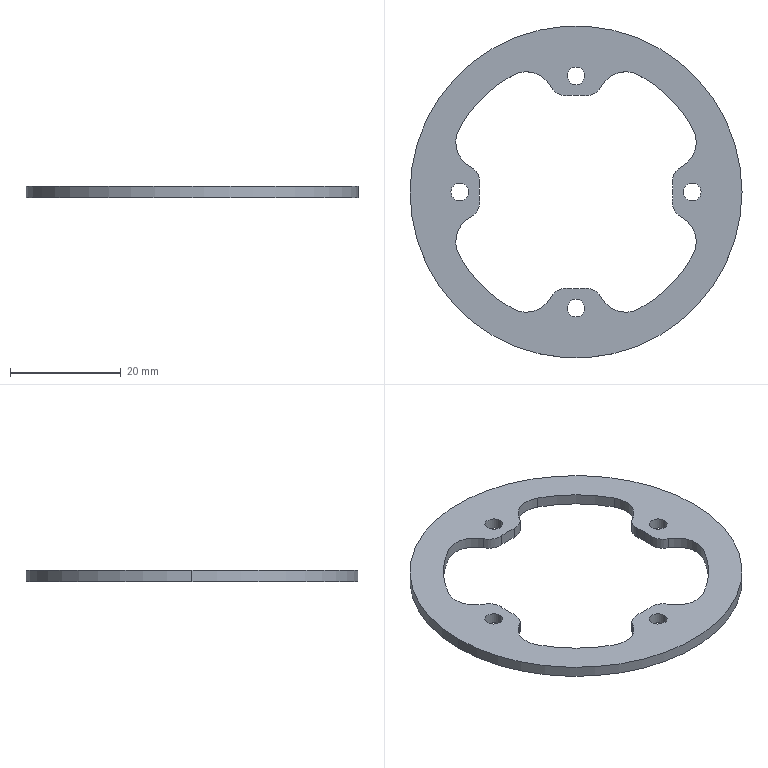Part | SolidWorks | features ICE 3, Extrusion 1, Fillet 1 | 1 solid | 41 faces | box 60 x 60 x 2 mm | volume 2571 mm3 | cylinder 39 | plane 2 | commonest cylinder face diameters 6 x10 10 x10 3.2 x8 35 x5 48 x4 60 x2
STEP:
#1=CARTESIAN_POINT('',(-17.412,1.896,0.));
#2=VERTEX_POINT('',#1);
#3=CARTESIAN_POINT('',(-17.425,1.619,0.));
#4=VERTEX_POINT('',#3);
#5=CARTESIAN_POINT('',(-20.412,1.896,0.));
#6=DIRECTION('',(0.,0.,-1.));
#7=DIRECTION('',(1.,0.,0.));
#8=AXIS2_PLACEMENT_3D('',#5,#6,#7);
#9=CIRCLE('',#8,3.);
#10=EDGE_CURVE('',#2,#4,#9,.T.);
#11=ORIENTED_EDGE('',*,*,#10,.F.);
#12=CARTESIAN_POINT('',(-17.412,1.896,2.));
#13=VERTEX_POINT('',#12);
#14=CARTESIAN_POINT('',(-17.412,1.896,2.));
#15=DIRECTION('',(0.,0.,1.));
#16=VECTOR('',#15,1000.);
#17=LINE('',#14,#16);
#18=EDGE_CURVE('',#2,#13,#17,.T.);
#19=ORIENTED_EDGE('',*,*,#18,.T.);
#20=CARTESIAN_POINT('',(-17.425,1.619,2.));
#21=VERTEX_POINT('',#20);
#22=CARTESIAN_POINT('',(-20.412,1.896,2.));
#23=DIRECTION('',(0.,0.,1.));
#24=DIRECTION('',(1.,0.,0.));
#25=AXIS2_PLACEMENT_3D('',#22,#23,#24);
#26=CIRCLE('',#25,3.);
#27=EDGE_CURVE('',#21,#13,#26,.T.);
#28=ORIENTED_EDGE('',*,*,#27,.F.);
#29=CARTESIAN_POINT('',(-17.425,1.619,-8.));
#30=DIRECTION('',(0.,0.,1.));
#31=VECTOR('',#30,1000.);
#32=LINE('',#29,#31);
#33=EDGE_CURVE('',#4,#21,#32,.T.);
#34=ORIENTED_EDGE('',*,*,#33,.F.);
#35=EDGE_LOOP('',(#11,#19,#28,#34));
#36=FACE_OUTER_BOUND('',#35,.T.);
#37=CARTESIAN_POINT('',(-20.412,1.896,2.));
#38=DIRECTION('',(0.,0.,1.));
#39=DIRECTION('',(1.,0.,0.));
#40=AXIS2_PLACEMENT_3D('',#37,#38,#39);
#41=CYLINDRICAL_SURFACE('',#40,3.);
#42=ADVANCED_FACE('',(#36),#41,.T.);
#43=CARTESIAN_POINT('',(17.412,1.896,2.));
#44=VERTEX_POINT('',#43);
#45=CARTESIAN_POINT('',(17.425,1.619,2.));
#46=VERTEX_POINT('',#45);
#47=CARTESIAN_POINT('',(20.412,1.896,2.));
#48=DIRECTION('',(0.,0.,1.));
#49=DIRECTION('',(1.,0.,0.));
#50=AXIS2_PLACEMENT_3D('',#47,#48,#49);
#51=CIRCLE('',#50,3.);
#52=EDGE_CURVE('',#44,#46,#51,.T.);
#53=ORIENTED_EDGE('',*,*,#52,.F.);
#54=CARTESIAN_POINT('',(17.412,1.896,0.));
#55=VERTEX_POINT('',#54);
#56=CARTESIAN_POINT('',(17.412,1.896,2.));
#57=DIRECTION('',(0.,0.,-1.));
#58=VECTOR('',#57,1000.);
#59=LINE('',#56,#58);
#60=EDGE_CURVE('',#44,#55,#59,.T.);
#61=ORIENTED_EDGE('',*,*,#60,.T.);
#62=CARTESIAN_POINT('',(17.425,1.619,0.));
#63=VERTEX_POINT('',#62);
#64=CARTESIAN_POINT('',(20.412,1.896,0.));
#65=DIRECTION('',(0.,0.,-1.));
#66=DIRECTION('',(1.,0.,0.));
#67=AXIS2_PLACEMENT_3D('',#64,#65,#66);
#68=CIRCLE('',#67,3.);
#69=EDGE_CURVE('',#63,#55,#68,.T.);
#70=ORIENTED_EDGE('',*,*,#69,.F.);
#71=CARTESIAN_POINT('',(17.425,1.619,-8.));
#72=DIRECTION('',(0.,0.,-1.));
#73=VECTOR('',#72,1000.);
#74=LINE('',#71,#73);
#75=EDGE_CURVE('',#46,#63,#74,.T.);
#76=ORIENTED_EDGE('',*,*,#75,.F.);
#77=EDGE_LOOP('',(#53,#61,#70,#76));
#78=FACE_OUTER_BOUND('',#77,.T.);
#79=CARTESIAN_POINT('',(20.412,1.896,2.));
#80=DIRECTION('',(0.,0.,-1.));
#81=DIRECTION('',(-1.,0.,0.));
#82=AXIS2_PLACEMENT_3D('',#79,#80,#81);
#83=CYLINDRICAL_SURFACE('',#82,3.);
#84=ADVANCED_FACE('',(#78),#83,.T.);
#85=CARTESIAN_POINT('',(17.5,0.,0.));
#86=VERTEX_POINT('',#85);
#87=CARTESIAN_POINT('',(0.,0.,0.));
#88=DIRECTION('',(0.,0.,1.));
#89=DIRECTION('',(1.,0.,0.));
#90=AXIS2_PLACEMENT_3D('',#87,#88,#89);
#91=CIRCLE('',#90,17.5);
#92=EDGE_CURVE('',#86,#63,#91,.T.);
#93=ORIENTED_EDGE('',*,*,#92,.F.);
#94=CARTESIAN_POINT('',(17.5,0.,2.));
#95=VERTEX_POINT('',#94);
#96=CARTESIAN_POINT('',(17.5,0.,-8.));
#97=DIRECTION('',(0.,0.,1.));
#98=VECTOR('',#97,1000.);
#99=LINE('',#96,#98);
#100=EDGE_CURVE('',#86,#95,#99,.T.);
#101=ORIENTED_EDGE('',*,*,#100,.T.);
#102=CARTESIAN_POINT('',(0.,0.,2.));
#103=DIRECTION('',(0.,0.,1.));
#104=DIRECTION('',(1.,0.,0.));
#105=AXIS2_PLACEMENT_3D('',#102,#103,#104);
#106=CIRCLE('',#105,17.5);
#107=EDGE_CURVE('',#95,#46,#106,.T.);
#108=ORIENTED_EDGE('',*,*,#107,.T.);
#109=ORIENTED_EDGE('',*,*,#75,.T.);
#110=EDGE_LOOP('',(#93,#101,#108,#109));
#111=FACE_OUTER_BOUND('',#110,.T.);
#112=CARTESIAN_POINT('',(0.,0.,-8.));
#113=DIRECTION('',(0.,0.,1.));
#114=DIRECTION('',(1.,0.,0.));
#115=AXIS2_PLACEMENT_3D('',#112,#113,#114);
#116=CYLINDRICAL_SURFACE('',#115,17.5);
#117=ADVANCED_FACE('',(#111),#116,.F.);
#118=CARTESIAN_POINT('',(-22.6,0.,0.));
#119=VERTEX_POINT('',#118);
#120=CARTESIAN_POINT('',(-19.4,0.,0.));
#121=VERTEX_POINT('',#120);
#122=CARTESIAN_POINT('',(-21.,0.,0.));
#123=DIRECTION('',(0.,0.,1.));
#124=DIRECTION('',(1.,0.,0.));
#125=AXIS2_PLACEMENT_3D('',#122,#123,#124);
#126=CIRCLE('',#125,1.6);
#127=EDGE_CURVE('',#119,#121,#126,.T.);
#128=ORIENTED_EDGE('',*,*,#127,.F.);
#129=CARTESIAN_POINT('',(-22.6,0.,2.));
#130=VERTEX_POINT('',#129);
#131=CARTESIAN_POINT('',(-22.6,0.,-8.));
#132=DIRECTION('',(0.,0.,1.));
#133=VECTOR('',#132,1000.);
#134=LINE('',#131,#133);
#135=EDGE_CURVE('',#119,#130,#134,.T.);
#136=ORIENTED_EDGE('',*,*,#135,.T.);
#137=CARTESIAN_POINT('',(-19.4,0.,2.));
#138=VERTEX_POINT('',#137);
#139=CARTESIAN_POINT('',(-21.,0.,2.));
#140=DIRECTION('',(0.,0.,1.));
#141=DIRECTION('',(1.,0.,0.));
#142=AXIS2_PLACEMENT_3D('',#139,#140,#141);
#143=CIRCLE('',#142,1.6);
#144=EDGE_CURVE('',#130,#138,#143,.T.);
#145=ORIENTED_EDGE('',*,*,#144,.T.);
#146=CARTESIAN_POINT('',(-19.4,0.,-8.));
#147=DIRECTION('',(0.,0.,1.));
#148=VECTOR('',#147,1000.);
#149=LINE('',#146,#148);
#150=EDGE_CURVE('',#121,#138,#149,.T.);
#151=ORIENTED_EDGE('',*,*,#150,.F.);
#152=EDGE_LOOP('',(#128,#136,#145,#151));
#153=FACE_OUTER_BOUND('',#152,.T.);
#154=CARTESIAN_POINT('',(-21.,0.,-8.));
#155=DIRECTION('',(0.,0.,1.));
#156=DIRECTION('',(1.,0.,0.));
#157=AXIS2_PLACEMENT_3D('',#154,#155,#156);
#158=CYLINDRICAL_SURFACE('',#157,1.6);
#159=ADVANCED_FACE('',(#153),#158,.F.);
#160=CARTESIAN_POINT('',(-1.6,21.,0.));
#161=VERTEX_POINT('',#160);
#162=CARTESIAN_POINT('',(1.6,21.,0.));
#163=VERTEX_POINT('',#162);
#164=CARTESIAN_POINT('',(0.,21.,0.));
#165=DIRECTION('',(0.,0.,1.));
#166=DIRECTION('',(1.,0.,0.));
#167=AXIS2_PLACEMENT_3D('',#164,#165,#166);
#168=CIRCLE('',#167,1.6);
#169=EDGE_CURVE('',#161,#163,#168,.T.);
#170=ORIENTED_EDGE('',*,*,#169,.F.);
#171=CARTESIAN_POINT('',(-1.6,21.,2.));
#172=VERTEX_POINT('',#171);
#173=CARTESIAN_POINT('',(-1.6,21.,-8.));
#174=DIRECTION('',(0.,0.,1.));
#175=VECTOR('',#174,1000.);
#176=LINE('',#173,#175);
#177=EDGE_CURVE('',#161,#172,#176,.T.);
#178=ORIENTED_EDGE('',*,*,#177,.T.);
#179=CARTESIAN_POINT('',(1.6,21.,2.));
#180=VERTEX_POINT('',#179);
#181=CARTESIAN_POINT('',(0.,21.,2.));
#182=DIRECTION('',(0.,0.,1.));
#183=DIRECTION('',(1.,0.,0.));
#184=AXIS2_PLACEMENT_3D('',#181,#182,#183);
#185=CIRCLE('',#184,1.6);
#186=EDGE_CURVE('',#172,#180,#185,.T.);
#187=ORIENTED_EDGE('',*,*,#186,.T.);
#188=CARTESIAN_POINT('',(1.6,21.,-8.));
#189=DIRECTION('',(0.,0.,1.));
#190=VECTOR('',#189,1000.);
#191=LINE('',#188,#190);
#192=EDGE_CURVE('',#163,#180,#191,.T.);
#193=ORIENTED_EDGE('',*,*,#192,.F.);
#194=EDGE_LOOP('',(#170,#178,#187,#193));
#195=FACE_OUTER_BOUND('',#194,.T.);
#196=CARTESIAN_POINT('',(0.,21.,-8.));
#197=DIRECTION('',(0.,0.,1.));
#198=DIRECTION('',(1.,0.,0.));
#199=AXIS2_PLACEMENT_3D('',#196,#197,#198);
#200=CYLINDRICAL_SURFACE('',#199,1.6);
#201=ADVANCED_FACE('',(#195),#200,.F.);
#202=CARTESIAN_POINT('',(19.4,0.,0.));
#203=VERTEX_POINT('',#202);
#204=CARTESIAN_POINT('',(22.6,0.,0.));
#205=VERTEX_POINT('',#204);
#206=CARTESIAN_POINT('',(21.,0.,0.));
#207=DIRECTION('',(0.,0.,1.));
#208=DIRECTION('',(1.,0.,0.));
#209=AXIS2_PLACEMENT_3D('',#206,#207,#208);
#210=CIRCLE('',#209,1.6);
#211=EDGE_CURVE('',#203,#205,#210,.T.);
#212=ORIENTED_EDGE('',*,*,#211,.F.);
#213=CARTESIAN_POINT('',(19.4,0.,2.));
#214=VERTEX_POINT('',#213);
#215=CARTESIAN_POINT('',(19.4,0.,-8.));
#216=DIRECTION('',(0.,0.,1.));
#217=VECTOR('',#216,1000.);
#218=LINE('',#215,#217);
#219=EDGE_CURVE('',#203,#214,#218,.T.);
#220=ORIENTED_EDGE('',*,*,#219,.T.);
#221=CARTESIAN_POINT('',(22.6,0.,2.));
#222=VERTEX_POINT('',#221);
#223=CARTESIAN_POINT('',(21.,0.,2.));
#224=DIRECTION('',(0.,0.,1.));
#225=DIRECTION('',(1.,0.,0.));
#226=AXIS2_PLACEMENT_3D('',#223,#224,#225);
#227=CIRCLE('',#226,1.6);
#228=EDGE_CURVE('',#214,#222,#227,.T.);
#229=ORIENTED_EDGE('',*,*,#228,.T.);
#230=CARTESIAN_POINT('',(22.6,0.,-8.));
#231=DIRECTION('',(0.,0.,1.));
#232=VECTOR('',#231,1000.);
#233=LINE('',#230,#232);
#234=EDGE_CURVE('',#205,#222,#233,.T.);
#235=ORIENTED_EDGE('',*,*,#234,.F.);
#236=EDGE_LOOP('',(#212,#220,#229,#235));
#237=FACE_OUTER_BOUND('',#236,.T.);
#238=CARTESIAN_POINT('',(21.,0.,-8.));
#239=DIRECTION('',(0.,0.,1.));
#240=DIRECTION('',(1.,0.,0.));
#241=AXIS2_PLACEMENT_3D('',#238,#239,#240);
#242=CYLINDRICAL_SURFACE('',#241,1.6);
#243=ADVANCED_FACE('',(#237),#242,.F.);
#244=CARTESIAN_POINT('',(-1.6,-21.,0.));
#245=VERTEX_POINT('',#244);
#246=CARTESIAN_POINT('',(1.6,-21.,0.));
#247=VERTEX_POINT('',#246);
#248=CARTESIAN_POINT('',(0.,-21.,0.));
#249=DIRECTION('',(0.,0.,1.));
#250=DIRECTION('',(1.,0.,0.));
#251=AXIS2_PLACEMENT_3D('',#248,#249,#250);
#252=CIRCLE('',#251,1.6);
#253=EDGE_CURVE('',#245,#247,#252,.T.);
#254=ORIENTED_EDGE('',*,*,#253,.F.);
#255=CARTESIAN_POINT('',(-1.6,-21.,2.));
#256=VERTEX_POINT('',#255);
#257=CARTESIAN_POINT('',(-1.6,-21.,-8.));
#258=DIRECTION('',(0.,0.,1.));
#259=VECTOR('',#258,1000.);
#260=LINE('',#257,#259);
#261=EDGE_CURVE('',#245,#256,#260,.T.);
#262=ORIENTED_EDGE('',*,*,#261,.T.);
#263=CARTESIAN_POINT('',(1.6,-21.,2.));
#264=VERTEX_POINT('',#263);
#265=CARTESIAN_POINT('',(0.,-21.,2.));
#266=DIRECTION('',(0.,0.,1.));
#267=DIRECTION('',(1.,0.,0.));
#268=AXIS2_PLACEMENT_3D('',#265,#266,#267);
#269=CIRCLE('',#268,1.6);
#270=EDGE_CURVE('',#256,#264,#269,.T.);
#271=ORIENTED_EDGE('',*,*,#270,.T.);
#272=CARTESIAN_POINT('',(1.6,-21.,-8.));
#273=DIRECTION('',(0.,0.,1.));
#274=VECTOR('',#273,1000.);
#275=LINE('',#272,#274);
#276=EDGE_CURVE('',#247,#264,#275,.T.);
#277=ORIENTED_EDGE('',*,*,#276,.F.);
#278=EDGE_LOOP('',(#254,#262,#271,#277));
#279=FACE_OUTER_BOUND('',#278,.T.);
#280=CARTESIAN_POINT('',(0.,-21.,-8.));
#281=DIRECTION('',(0.,0.,1.));
#282=DIRECTION('',(1.,0.,0.));
#283=AXIS2_PLACEMENT_3D('',#280,#281,#282);
#284=CYLINDRICAL_SURFACE('',#283,1.6);
#285=ADVANCED_FACE('',(#279),#284,.F.);
#286=CARTESIAN_POINT('',(-19.033,-4.56,2.));
#287=VERTEX_POINT('',#286);
#288=CARTESIAN_POINT('',(-21.733,-9.,2.));
#289=VERTEX_POINT('',#288);
#290=CARTESIAN_POINT('',(-16.733,-9.,2.));
#291=DIRECTION('',(0.,0.,1.));
#292=DIRECTION('',(1.,0.,0.));
#293=AXIS2_PLACEMENT_3D('',#290,#291,#292);
#294=CIRCLE('',#293,5.);
#295=EDGE_CURVE('',#287,#289,#294,.T.);
#296=ORIENTED_EDGE('',*,*,#295,.T.);
#297=CARTESIAN_POINT('',(-21.733,-9.,0.));
#298=VERTEX_POINT('',#297);
#299=CARTESIAN_POINT('',(-21.733,-9.,2.));
#300=DIRECTION('',(0.,0.,-1.));
#301=VECTOR('',#300,1000.);
#302=LINE('',#299,#301);
#303=EDGE_CURVE('',#289,#298,#302,.T.);
#304=ORIENTED_EDGE('',*,*,#303,.T.);
#305=CARTESIAN_POINT('',(-19.033,-4.56,0.));
#306=VERTEX_POINT('',#305);
#307=CARTESIAN_POINT('',(-16.733,-9.,0.));
#308=DIRECTION('',(0.,0.,1.));
#309=DIRECTION('',(1.,0.,0.));
#310=AXIS2_PLACEMENT_3D('',#307,#308,#309);
#311=CIRCLE('',#310,5.);
#312=EDGE_CURVE('',#306,#298,#311,.T.);
#313=ORIENTED_EDGE('',*,*,#312,.F.);
#314=CARTESIAN_POINT('',(-19.033,-4.56,2.));
#315=DIRECTION('',(0.,0.,1.));
#316=VECTOR('',#315,1000.);
#317=LINE('',#314,#316);
#318=EDGE_CURVE('',#306,#287,#317,.T.);
#319=ORIENTED_EDGE('',*,*,#318,.T.);
#320=EDGE_LOOP('',(#296,#304,#313,#319));
#321=FACE_OUTER_BOUND('',#320,.T.);
#322=CARTESIAN_POINT('',(-16.733,-9.,2.));
#323=DIRECTION('',(0.,0.,-1.));
#324=DIRECTION('',(-1.,0.,0.));
#325=AXIS2_PLACEMENT_3D('',#322,#323,#324);
#326=CYLINDRICAL_SURFACE('',#325,5.);
#327=ADVANCED_FACE('',(#321),#326,.F.);
#328=CARTESIAN_POINT('',(-21.137,11.368,2.));
#329=VERTEX_POINT('',#328);
#330=CARTESIAN_POINT('',(-21.733,9.,2.));
#331=VERTEX_POINT('',#330);
#332=CARTESIAN_POINT('',(-16.733,9.,2.));
#333=DIRECTION('',(0.,0.,1.));
#334=DIRECTION('',(-1.,0.,0.));
#335=AXIS2_PLACEMENT_3D('',#332,#333,#334);
#336=CIRCLE('',#335,5.);
#337=EDGE_CURVE('',#329,#331,#336,.T.);
#338=ORIENTED_EDGE('',*,*,#337,.T.);
#339=CARTESIAN_POINT('',(-21.733,9.,0.));
#340=VERTEX_POINT('',#339);
#341=CARTESIAN_POINT('',(-21.733,9.,2.));
#342=DIRECTION('',(0.,0.,-1.));
#343=VECTOR('',#342,1000.);
#344=LINE('',#341,#343);
#345=EDGE_CURVE('',#331,#340,#344,.T.);
#346=ORIENTED_EDGE('',*,*,#345,.T.);
#347=CARTESIAN_POINT('',(-21.137,11.368,0.));
#348=VERTEX_POINT('',#347);
#349=CARTESIAN_POINT('',(-16.733,9.,0.));
#350=DIRECTION('',(0.,0.,1.));
#351=DIRECTION('',(-1.,0.,0.));
#352=AXIS2_PLACEMENT_3D('',#349,#350,#351);
#353=CIRCLE('',#352,5.);
#354=EDGE_CURVE('',#348,#340,#353,.T.);
#355=ORIENTED_EDGE('',*,*,#354,.F.);
#356=CARTESIAN_POINT('',(-21.137,11.368,2.));
#357=DIRECTION('',(0.,0.,-1.));
#358=VECTOR('',#357,1000.);
#359=LINE('',#356,#358);
#360=EDGE_CURVE('',#329,#348,#359,.T.);
#361=ORIENTED_EDGE('',*,*,#360,.F.);
#362=EDGE_LOOP('',(#338,#346,#355,#361));
#363=FACE_OUTER_BOUND('',#362,.T.);
#364=CARTESIAN_POINT('',(-16.733,9.,2.));
#365=DIRECTION('',(0.,0.,-1.));
#366=DIRECTION('',(-1.,0.,0.));
#367=AXIS2_PLACEMENT_3D('',#364,#365,#366);
#368=CYLINDRICAL_SURFACE('',#367,5.);
#369=ADVANCED_FACE('',(#363),#368,.F.);
#370=CARTESIAN_POINT('',(30.,0.,2.));
#371=VERTEX_POINT('',#370);
#372=CARTESIAN_POINT('',(-30.,0.,2.));
#373=VERTEX_POINT('',#372);
#374=CARTESIAN_POINT('',(0.,0.,2.));
#375=DIRECTION('',(0.,0.,1.));
#376=DIRECTION('',(1.,0.,0.));
#377=AXIS2_PLACEMENT_3D('',#374,#375,#376);
#378=CIRCLE('',#377,30.);
#379=EDGE_CURVE('',#371,#373,#378,.T.);
#380=ORIENTED_EDGE('',*,*,#379,.F.);
#381=CARTESIAN_POINT('',(30.,0.,0.));
#382=VERTEX_POINT('',#381);
#383=CARTESIAN_POINT('',(30.,0.,2.));
#384=DIRECTION('',(0.,0.,-1.));
#385=VECTOR('',#384,1000.);
#386=LINE('',#383,#385);
#387=EDGE_CURVE('',#371,#382,#386,.T.);
#388=ORIENTED_EDGE('',*,*,#387,.T.);
#389=CARTESIAN_POINT('',(-30.,0.,0.));
#390=VERTEX_POINT('',#389);
#391=CARTESIAN_POINT('',(0.,0.,0.));
#392=DIRECTION('',(0.,0.,1.));
#393=DIRECTION('',(1.,0.,0.));
#394=AXIS2_PLACEMENT_3D('',#391,#392,#393);
#395=CIRCLE('',#394,30.);
#396=EDGE_CURVE('',#382,#390,#395,.T.);
#397=ORIENTED_EDGE('',*,*,#396,.T.);
#398=CARTESIAN_POINT('',(-30.,0.,2.));
#399=DIRECTION('',(0.,0.,-1.));
#400=VECTOR('',#399,1000.);
#401=LINE('',#398,#400);
#402=EDGE_CURVE('',#373,#390,#401,.T.);
#403=ORIENTED_EDGE('',*,*,#402,.F.);
#404=EDGE_LOOP('',(#380,#388,#397,#403));
#405=FACE_OUTER_BOUND('',#404,.T.);
#406=CARTESIAN_POINT('',(0.,0.,2.));
#407=DIRECTION('',(0.,0.,-1.));
#408=DIRECTION('',(-1.,0.,0.));
#409=AXIS2_PLACEMENT_3D('',#406,#407,#408);
#410=CYLINDRICAL_SURFACE('',#409,30.);
#411=ADVANCED_FACE('',(#405),#410,.T.);
#412=CARTESIAN_POINT('',(17.425,-1.619,2.));
#413=VERTEX_POINT('',#412);
#414=CARTESIAN_POINT('',(0.,0.,2.));
#415=DIRECTION('',(0.,0.,1.));
#416=DIRECTION('',(1.,0.,0.));
#417=AXIS2_PLACEMENT_3D('',#414,#415,#416);
#418=CIRCLE('',#417,17.5);
#419=EDGE_CURVE('',#413,#95,#418,.T.);
#420=ORIENTED_EDGE('',*,*,#419,.F.);
#421=CARTESIAN_POINT('',(19.033,-4.56,2.));
#422=VERTEX_POINT('',#421);
#423=CARTESIAN_POINT('',(20.412,-1.896,2.));
#424=DIRECTION('',(0.,0.,1.));
#425=DIRECTION('',(1.,0.,0.));
#426=AXIS2_PLACEMENT_3D('',#423,#424,#425);
#427=CIRCLE('',#426,3.);
#428=EDGE_CURVE('',#413,#422,#427,.T.);
#429=ORIENTED_EDGE('',*,*,#428,.T.);
#430=CARTESIAN_POINT('',(21.137,-11.368,2.));
#431=VERTEX_POINT('',#430);
#432=CARTESIAN_POINT('',(16.733,-9.,2.));
#433=DIRECTION('',(0.,0.,1.));
#434=DIRECTION('',(-1.,0.,0.));
#435=AXIS2_PLACEMENT_3D('',#432,#433,#434);
#436=CIRCLE('',#435,5.);
#437=EDGE_CURVE('',#431,#422,#436,.T.);
#438=ORIENTED_EDGE('',*,*,#437,.F.);
#439=CARTESIAN_POINT('',(11.368,-21.137,2.));
#440=VERTEX_POINT('',#439);
#441=CARTESIAN_POINT('',(0.,0.,2.));
#442=DIRECTION('',(0.,0.,1.));
#443=DIRECTION('',(1.,0.,0.));
#444=AXIS2_PLACEMENT_3D('',#441,#442,#443);
#445=CIRCLE('',#444,24.);
#446=EDGE_CURVE('',#440,#431,#445,.T.);
#447=ORIENTED_EDGE('',*,*,#446,.F.);
#448=CARTESIAN_POINT('',(4.56,-19.033,2.));
#449=VERTEX_POINT('',#448);
#450=CARTESIAN_POINT('',(9.,-16.733,2.));
#451=DIRECTION('',(0.,0.,1.));
#452=DIRECTION('',(1.,0.,0.));
#453=AXIS2_PLACEMENT_3D('',#450,#451,#452);
#454=CIRCLE('',#453,5.);
#455=EDGE_CURVE('',#449,#440,#454,.T.);
#456=ORIENTED_EDGE('',*,*,#455,.F.);
#457=CARTESIAN_POINT('',(1.619,-17.425,2.));
#458=VERTEX_POINT('',#457);
#459=CARTESIAN_POINT('',(1.896,-20.412,2.));
#460=DIRECTION('',(0.,0.,1.));
#461=DIRECTION('',(1.,0.,0.));
#462=AXIS2_PLACEMENT_3D('',#459,#460,#461);
#463=CIRCLE('',#462,3.);
#464=EDGE_CURVE('',#449,#458,#463,.T.);
#465=ORIENTED_EDGE('',*,*,#464,.T.);
#466=CARTESIAN_POINT('',(-1.619,-17.425,2.));
#467=VERTEX_POINT('',#466);
#468=CARTESIAN_POINT('',(0.,0.,2.));
#469=DIRECTION('',(0.,0.,1.));
#470=DIRECTION('',(1.,0.,0.));
#471=AXIS2_PLACEMENT_3D('',#468,#469,#470);
#472=CIRCLE('',#471,17.5);
#473=EDGE_CURVE('',#467,#458,#472,.T.);
#474=ORIENTED_EDGE('',*,*,#473,.F.);
#475=CARTESIAN_POINT('',(-4.56,-19.033,2.));
#476=VERTEX_POINT('',#475);
#477=CARTESIAN_POINT('',(-1.896,-20.412,2.));
#478=DIRECTION('',(0.,0.,1.));
#479=DIRECTION('',(1.,0.,0.));
#480=AXIS2_PLACEMENT_3D('',#477,#478,#479);
#481=CIRCLE('',#480,3.);
#482=EDGE_CURVE('',#467,#476,#481,.T.);
#483=ORIENTED_EDGE('',*,*,#482,.T.);
#484=CARTESIAN_POINT('',(-11.368,-21.137,2.));
#485=VERTEX_POINT('',#484);
#486=CARTESIAN_POINT('',(-9.,-16.733,2.));
#487=DIRECTION('',(0.,0.,1.));
#488=DIRECTION('',(-1.,0.,0.));
#489=AXIS2_PLACEMENT_3D('',#486,#487,#488);
#490=CIRCLE('',#489,5.);
#491=EDGE_CURVE('',#485,#476,#490,.T.);
#492=ORIENTED_EDGE('',*,*,#491,.F.);
#493=CARTESIAN_POINT('',(-21.137,-11.368,2.));
#494=VERTEX_POINT('',#493);
#495=CARTESIAN_POINT('',(0.,0.,2.));
#496=DIRECTION('',(0.,0.,1.));
#497=DIRECTION('',(1.,0.,0.));
#498=AXIS2_PLACEMENT_3D('',#495,#496,#497);
#499=CIRCLE('',#498,24.);
#500=EDGE_CURVE('',#494,#485,#499,.T.);
#501=ORIENTED_EDGE('',*,*,#500,.F.);
#502=CARTESIAN_POINT('',(-16.733,-9.,2.));
#503=DIRECTION('',(0.,0.,1.));
#504=DIRECTION('',(1.,0.,0.));
#505=AXIS2_PLACEMENT_3D('',#502,#503,#504);
#506=CIRCLE('',#505,5.);
#507=EDGE_CURVE('',#289,#494,#506,.T.);
#508=ORIENTED_EDGE('',*,*,#507,.F.);
#509=ORIENTED_EDGE('',*,*,#295,.F.);
#510=CARTESIAN_POINT('',(-17.425,-1.619,2.));
#511=VERTEX_POINT('',#510);
#512=CARTESIAN_POINT('',(-20.412,-1.896,2.));
#513=DIRECTION('',(0.,0.,1.));
#514=DIRECTION('',(1.,0.,0.));
#515=AXIS2_PLACEMENT_3D('',#512,#513,#514);
#516=CIRCLE('',#515,3.);
#517=EDGE_CURVE('',#287,#511,#516,.T.);
#518=ORIENTED_EDGE('',*,*,#517,.T.);
#519=CARTESIAN_POINT('',(0.,0.,2.));
#520=DIRECTION('',(0.,0.,1.));
#521=DIRECTION('',(1.,0.,0.));
#522=AXIS2_PLACEMENT_3D('',#519,#520,#521);
#523=CIRCLE('',#522,17.5);
#524=EDGE_CURVE('',#21,#511,#523,.T.);
#525=ORIENTED_EDGE('',*,*,#524,.F.);
#526=ORIENTED_EDGE('',*,*,#27,.T.);
#527=CARTESIAN_POINT('',(-19.033,4.56,2.));
#528=VERTEX_POINT('',#527);
#529=CARTESIAN_POINT('',(-20.412,1.896,2.));
#530=DIRECTION('',(0.,0.,1.));
#531=DIRECTION('',(1.,0.,0.));
#532=AXIS2_PLACEMENT_3D('',#529,#530,#531);
#533=CIRCLE('',#532,3.);
#534=EDGE_CURVE('',#13,#528,#533,.T.);
#535=ORIENTED_EDGE('',*,*,#534,.T.);
#536=CARTESIAN_POINT('',(-16.733,9.,2.));
#537=DIRECTION('',(0.,0.,1.));
#538=DIRECTION('',(-1.,0.,0.));
#539=AXIS2_PLACEMENT_3D('',#536,#537,#538);
#540=CIRCLE('',#539,5.);
#541=EDGE_CURVE('',#331,#528,#540,.T.);
#542=ORIENTED_EDGE('',*,*,#541,.F.);
#543=ORIENTED_EDGE('',*,*,#337,.F.);
#544=CARTESIAN_POINT('',(-11.368,21.137,2.));
#545=VERTEX_POINT('',#544);
#546=CARTESIAN_POINT('',(0.,0.,2.));
#547=DIRECTION('',(0.,0.,1.));
#548=DIRECTION('',(1.,0.,0.));
#549=AXIS2_PLACEMENT_3D('',#546,#547,#548);
#550=CIRCLE('',#549,24.);
#551=EDGE_CURVE('',#545,#329,#550,.T.);
#552=ORIENTED_EDGE('',*,*,#551,.F.);
#553=CARTESIAN_POINT('',(-4.56,19.033,2.));
#554=VERTEX_POINT('',#553);
#555=CARTESIAN_POINT('',(-9.,16.733,2.));
#556=DIRECTION('',(0.,0.,1.));
#557=DIRECTION('',(1.,0.,0.));
#558=AXIS2_PLACEMENT_3D('',#555,#556,#557);
#559=CIRCLE('',#558,5.);
#560=EDGE_CURVE('',#554,#545,#559,.T.);
#561=ORIENTED_EDGE('',*,*,#560,.F.);
#562=CARTESIAN_POINT('',(-1.619,17.425,2.));
#563=VERTEX_POINT('',#562);
#564=CARTESIAN_POINT('',(-1.896,20.412,2.));
#565=DIRECTION('',(0.,0.,1.));
#566=DIRECTION('',(1.,0.,0.));
#567=AXIS2_PLACEMENT_3D('',#564,#565,#566);
#568=CIRCLE('',#567,3.);
#569=EDGE_CURVE('',#554,#563,#568,.T.);
#570=ORIENTED_EDGE('',*,*,#569,.T.);
#571=CARTESIAN_POINT('',(1.619,17.425,2.));
#572=VERTEX_POINT('',#571);
#573=CARTESIAN_POINT('',(0.,0.,2.));
#574=DIRECTION('',(0.,0.,1.));
#575=DIRECTION('',(1.,0.,0.));
#576=AXIS2_PLACEMENT_3D('',#573,#574,#575);
#577=CIRCLE('',#576,17.5);
#578=EDGE_CURVE('',#572,#563,#577,.T.);
#579=ORIENTED_EDGE('',*,*,#578,.F.);
#580=CARTESIAN_POINT('',(4.56,19.033,2.));
#581=VERTEX_POINT('',#580);
#582=CARTESIAN_POINT('',(1.896,20.412,2.));
#583=DIRECTION('',(0.,0.,1.));
#584=DIRECTION('',(1.,0.,0.));
#585=AXIS2_PLACEMENT_3D('',#582,#583,#584);
#586=CIRCLE('',#585,3.);
#587=EDGE_CURVE('',#572,#581,#586,.T.);
#588=ORIENTED_EDGE('',*,*,#587,.T.);
#589=CARTESIAN_POINT('',(11.368,21.137,2.));
#590=VERTEX_POINT('',#589);
#591=CARTESIAN_POINT('',(9.,16.733,2.));
#592=DIRECTION('',(0.,0.,1.));
#593=DIRECTION('',(-1.,0.,0.));
#594=AXIS2_PLACEMENT_3D('',#591,#592,#593);
#595=CIRCLE('',#594,5.);
#596=EDGE_CURVE('',#590,#581,#595,.T.);
#597=ORIENTED_EDGE('',*,*,#596,.F.);
#598=CARTESIAN_POINT('',(21.137,11.368,2.));
#599=VERTEX_POINT('',#598);
#600=CARTESIAN_POINT('',(0.,0.,2.));
#601=DIRECTION('',(0.,0.,1.));
#602=DIRECTION('',(1.,0.,0.));
#603=AXIS2_PLACEMENT_3D('',#600,#601,#602);
#604=CIRCLE('',#603,24.);
#605=EDGE_CURVE('',#599,#590,#604,.T.);
#606=ORIENTED_EDGE('',*,*,#605,.F.);
#607=CARTESIAN_POINT('',(19.033,4.56,2.));
#608=VERTEX_POINT('',#607);
#609=CARTESIAN_POINT('',(16.733,9.,2.));
#610=DIRECTION('',(0.,0.,1.));
#611=DIRECTION('',(1.,0.,0.));
#612=AXIS2_PLACEMENT_3D('',#609,#610,#611);
#613=CIRCLE('',#612,5.);
#614=EDGE_CURVE('',#608,#599,#613,.T.);
#615=ORIENTED_EDGE('',*,*,#614,.F.);
#616=CARTESIAN_POINT('',(20.412,1.896,2.));
#617=DIRECTION('',(0.,0.,1.));
#618=DIRECTION('',(1.,0.,0.));
#619=AXIS2_PLACEMENT_3D('',#616,#617,#618);
#620=CIRCLE('',#619,3.);
#621=EDGE_CURVE('',#608,#44,#620,.T.);
#622=ORIENTED_EDGE('',*,*,#621,.T.);
#623=ORIENTED_EDGE('',*,*,#52,.T.);
#624=ORIENTED_EDGE('',*,*,#107,.F.);
#625=EDGE_LOOP('',(#420,#429,#438,#447,#456,#465,#474,#483,#492,#501,#508,#509,#518,#525,#526,#535,#542,#543,#552,#561,#570,#579,#588,#597,#606,#615,#622,#623,#624));
#626=FACE_BOUND('',#625,.T.);
#627=CARTESIAN_POINT('',(-21.,0.,2.));
#628=DIRECTION('',(0.,0.,1.));
#629=DIRECTION('',(1.,0.,0.));
#630=AXIS2_PLACEMENT_3D('',#627,#628,#629);
#631=CIRCLE('',#630,1.6);
#632=EDGE_CURVE('',#138,#130,#631,.T.);
#633=ORIENTED_EDGE('',*,*,#632,.F.);
#634=ORIENTED_EDGE('',*,*,#144,.F.);
#635=EDGE_LOOP('',(#633,#634));
#636=FACE_BOUND('',#635,.T.);
#637=CARTESIAN_POINT('',(0.,21.,2.));
#638=DIRECTION('',(0.,0.,1.));
#639=DIRECTION('',(1.,0.,0.));
#640=AXIS2_PLACEMENT_3D('',#637,#638,#639);
#641=CIRCLE('',#640,1.6);
#642=EDGE_CURVE('',#180,#172,#641,.T.);
#643=ORIENTED_EDGE('',*,*,#642,.F.);
#644=ORIENTED_EDGE('',*,*,#186,.F.);
#645=EDGE_LOOP('',(#643,#644));
#646=FACE_BOUND('',#645,.T.);
#647=CARTESIAN_POINT('',(21.,0.,2.));
#648=DIRECTION('',(0.,0.,1.));
#649=DIRECTION('',(1.,0.,0.));
#650=AXIS2_PLACEMENT_3D('',#647,#648,#649);
#651=CIRCLE('',#650,1.6);
#652=EDGE_CURVE('',#222,#214,#651,.T.);
#653=ORIENTED_EDGE('',*,*,#652,.F.);
#654=ORIENTED_EDGE('',*,*,#228,.F.);
#655=EDGE_LOOP('',(#653,#654));
#656=FACE_BOUND('',#655,.T.);
#657=CARTESIAN_POINT('',(0.,-21.,2.));
#658=DIRECTION('',(0.,0.,1.));
#659=DIRECTION('',(1.,0.,0.));
#660=AXIS2_PLACEMENT_3D('',#657,#658,#659);
#661=CIRCLE('',#660,1.6);
#662=EDGE_CURVE('',#264,#256,#661,.T.);
#663=ORIENTED_EDGE('',*,*,#662,.F.);
#664=ORIENTED_EDGE('',*,*,#270,.F.);
#665=EDGE_LOOP('',(#663,#664));
#666=FACE_BOUND('',#665,.T.);
#667=CARTESIAN_POINT('',(0.,0.,2.));
#668=DIRECTION('',(0.,0.,1.));
#669=DIRECTION('',(1.,0.,0.));
#670=AXIS2_PLACEMENT_3D('',#667,#668,#669);
#671=CIRCLE('',#670,30.);
#672=EDGE_CURVE('',#373,#371,#671,.T.);
#673=ORIENTED_EDGE('',*,*,#672,.T.);
#674=ORIENTED_EDGE('',*,*,#379,.T.);
#675=EDGE_LOOP('',(#673,#674));
#676=FACE_OUTER_BOUND('',#675,.T.);
#677=CARTESIAN_POINT('',(0.,0.,2.));
#678=DIRECTION('',(0.,0.,1.));
#679=DIRECTION('',(1.,0.,0.));
#680=AXIS2_PLACEMENT_3D('',#677,#678,#679);
#681=PLANE('',#680);
#682=ADVANCED_FACE('',(#626,#636,#646,#656,#666,#676),#681,.T.);
#683=CARTESIAN_POINT('',(-21.,0.,0.));
#684=DIRECTION('',(0.,0.,1.));
#685=DIRECTION('',(1.,0.,0.));
#686=AXIS2_PLACEMENT_3D('',#683,#684,#685);
#687=CIRCLE('',#686,1.6);
#688=EDGE_CURVE('',#121,#119,#687,.T.);
#689=ORIENTED_EDGE('',*,*,#688,.T.);
#690=ORIENTED_EDGE('',*,*,#127,.T.);
#691=EDGE_LOOP('',(#689,#690));
#692=FACE_BOUND('',#691,.T.);
#693=CARTESIAN_POINT('',(0.,21.,0.));
#694=DIRECTION('',(0.,0.,1.));
#695=DIRECTION('',(1.,0.,0.));
#696=AXIS2_PLACEMENT_3D('',#693,#694,#695);
#697=CIRCLE('',#696,1.6);
#698=EDGE_CURVE('',#163,#161,#697,.T.);
#699=ORIENTED_EDGE('',*,*,#698,.T.);
#700=ORIENTED_EDGE('',*,*,#169,.T.);
#701=EDGE_LOOP('',(#699,#700));
#702=FACE_BOUND('',#701,.T.);
#703=CARTESIAN_POINT('',(21.,0.,0.));
#704=DIRECTION('',(0.,0.,1.));
#705=DIRECTION('',(1.,0.,0.));
#706=AXIS2_PLACEMENT_3D('',#703,#704,#705);
#707=CIRCLE('',#706,1.6);
#708=EDGE_CURVE('',#205,#203,#707,.T.);
#709=ORIENTED_EDGE('',*,*,#708,.T.);
#710=ORIENTED_EDGE('',*,*,#211,.T.);
#711=EDGE_LOOP('',(#709,#710));
#712=FACE_BOUND('',#711,.T.);
#713=CARTESIAN_POINT('',(0.,-21.,0.));
#714=DIRECTION('',(0.,0.,1.));
#715=DIRECTION('',(1.,0.,0.));
#716=AXIS2_PLACEMENT_3D('',#713,#714,#715);
#717=CIRCLE('',#716,1.6);
#718=EDGE_CURVE('',#247,#245,#717,.T.);
#719=ORIENTED_EDGE('',*,*,#718,.T.);
#720=ORIENTED_EDGE('',*,*,#253,.T.);
#721=EDGE_LOOP('',(#719,#720));
#722=FACE_BOUND('',#721,.T.);
#723=CARTESIAN_POINT('',(0.,0.,0.));
#724=DIRECTION('',(0.,0.,1.));
#725=DIRECTION('',(1.,0.,0.));
#726=AXIS2_PLACEMENT_3D('',#723,#724,#725);
#727=CIRCLE('',#726,30.);
#728=EDGE_CURVE('',#390,#382,#727,.T.);
#729=ORIENTED_EDGE('',*,*,#728,.F.);
#730=ORIENTED_EDGE('',*,*,#396,.F.);
#731=EDGE_LOOP('',(#729,#730));
#732=FACE_OUTER_BOUND('',#731,.T.);
#733=CARTESIAN_POINT('',(21.137,-11.368,0.));
#734=VERTEX_POINT('',#733);
#735=CARTESIAN_POINT('',(19.033,-4.56,0.));
#736=VERTEX_POINT('',#735);
#737=CARTESIAN_POINT('',(16.733,-9.,0.));
#738=DIRECTION('',(0.,0.,1.));
#739=DIRECTION('',(-1.,0.,0.));
#740=AXIS2_PLACEMENT_3D('',#737,#738,#739);
#741=CIRCLE('',#740,5.);
#742=EDGE_CURVE('',#734,#736,#741,.T.);
#743=ORIENTED_EDGE('',*,*,#742,.T.);
#744=CARTESIAN_POINT('',(17.425,-1.619,0.));
#745=VERTEX_POINT('',#744);
#746=CARTESIAN_POINT('',(20.412,-1.896,0.));
#747=DIRECTION('',(0.,0.,-1.));
#748=DIRECTION('',(1.,0.,0.));
#749=AXIS2_PLACEMENT_3D('',#746,#747,#748);
#750=CIRCLE('',#749,3.);
#751=EDGE_CURVE('',#736,#745,#750,.T.);
#752=ORIENTED_EDGE('',*,*,#751,.T.);
#753=CARTESIAN_POINT('',(0.,0.,0.));
#754=DIRECTION('',(0.,0.,1.));
#755=DIRECTION('',(1.,0.,0.));
#756=AXIS2_PLACEMENT_3D('',#753,#754,#755);
#757=CIRCLE('',#756,17.5);
#758=EDGE_CURVE('',#745,#86,#757,.T.);
#759=ORIENTED_EDGE('',*,*,#758,.T.);
#760=ORIENTED_EDGE('',*,*,#92,.T.);
#761=ORIENTED_EDGE('',*,*,#69,.T.);
#762=CARTESIAN_POINT('',(19.033,4.56,0.));
#763=VERTEX_POINT('',#762);
#764=CARTESIAN_POINT('',(20.412,1.896,0.));
#765=DIRECTION('',(0.,0.,-1.));
#766=DIRECTION('',(1.,0.,0.));
#767=AXIS2_PLACEMENT_3D('',#764,#765,#766);
#768=CIRCLE('',#767,3.);
#769=EDGE_CURVE('',#55,#763,#768,.T.);
#770=ORIENTED_EDGE('',*,*,#769,.T.);
#771=CARTESIAN_POINT('',(21.137,11.368,0.));
#772=VERTEX_POINT('',#771);
#773=CARTESIAN_POINT('',(16.733,9.,0.));
#774=DIRECTION('',(0.,0.,1.));
#775=DIRECTION('',(1.,0.,0.));
#776=AXIS2_PLACEMENT_3D('',#773,#774,#775);
#777=CIRCLE('',#776,5.);
#778=EDGE_CURVE('',#763,#772,#777,.T.);
#779=ORIENTED_EDGE('',*,*,#778,.T.);
#780=CARTESIAN_POINT('',(11.368,21.137,0.));
#781=VERTEX_POINT('',#780);
#782=CARTESIAN_POINT('',(0.,0.,0.));
#783=DIRECTION('',(0.,0.,1.));
#784=DIRECTION('',(1.,0.,0.));
#785=AXIS2_PLACEMENT_3D('',#782,#783,#784);
#786=CIRCLE('',#785,24.);
#787=EDGE_CURVE('',#772,#781,#786,.T.);
#788=ORIENTED_EDGE('',*,*,#787,.T.);
#789=CARTESIAN_POINT('',(4.56,19.033,0.));
#790=VERTEX_POINT('',#789);
#791=CARTESIAN_POINT('',(9.,16.733,0.));
#792=DIRECTION('',(0.,0.,1.));
#793=DIRECTION('',(-1.,0.,0.));
#794=AXIS2_PLACEMENT_3D('',#791,#792,#793);
#795=CIRCLE('',#794,5.);
#796=EDGE_CURVE('',#781,#790,#795,.T.);
#797=ORIENTED_EDGE('',*,*,#796,.T.);
#798=CARTESIAN_POINT('',(1.619,17.425,0.));
#799=VERTEX_POINT('',#798);
#800=CARTESIAN_POINT('',(1.896,20.412,0.));
#801=DIRECTION('',(0.,0.,-1.));
#802=DIRECTION('',(1.,0.,0.));
#803=AXIS2_PLACEMENT_3D('',#800,#801,#802);
#804=CIRCLE('',#803,3.);
#805=EDGE_CURVE('',#790,#799,#804,.T.);
#806=ORIENTED_EDGE('',*,*,#805,.T.);
#807=CARTESIAN_POINT('',(-1.619,17.425,0.));
#808=VERTEX_POINT('',#807);
#809=CARTESIAN_POINT('',(0.,0.,0.));
#810=DIRECTION('',(0.,0.,1.));
#811=DIRECTION('',(1.,0.,0.));
#812=AXIS2_PLACEMENT_3D('',#809,#810,#811);
#813=CIRCLE('',#812,17.5);
#814=EDGE_CURVE('',#799,#808,#813,.T.);
#815=ORIENTED_EDGE('',*,*,#814,.T.);
#816=CARTESIAN_POINT('',(-4.56,19.033,0.));
#817=VERTEX_POINT('',#816);
#818=CARTESIAN_POINT('',(-1.896,20.412,0.));
#819=DIRECTION('',(0.,0.,-1.));
#820=DIRECTION('',(1.,0.,0.));
#821=AXIS2_PLACEMENT_3D('',#818,#819,#820);
#822=CIRCLE('',#821,3.);
#823=EDGE_CURVE('',#808,#817,#822,.T.);
#824=ORIENTED_EDGE('',*,*,#823,.T.);
#825=CARTESIAN_POINT('',(-11.368,21.137,0.));
#826=VERTEX_POINT('',#825);
#827=CARTESIAN_POINT('',(-9.,16.733,0.));
#828=DIRECTION('',(0.,0.,1.));
#829=DIRECTION('',(1.,0.,0.));
#830=AXIS2_PLACEMENT_3D('',#827,#828,#829);
#831=CIRCLE('',#830,5.);
#832=EDGE_CURVE('',#817,#826,#831,.T.);
#833=ORIENTED_EDGE('',*,*,#832,.T.);
#834=CARTESIAN_POINT('',(0.,0.,0.));
#835=DIRECTION('',(0.,0.,1.));
#836=DIRECTION('',(1.,0.,0.));
#837=AXIS2_PLACEMENT_3D('',#834,#835,#836);
#838=CIRCLE('',#837,24.);
#839=EDGE_CURVE('',#826,#348,#838,.T.);
#840=ORIENTED_EDGE('',*,*,#839,.T.);
#841=ORIENTED_EDGE('',*,*,#354,.T.);
#842=CARTESIAN_POINT('',(-19.033,4.56,0.));
#843=VERTEX_POINT('',#842);
#844=CARTESIAN_POINT('',(-16.733,9.,0.));
#845=DIRECTION('',(0.,0.,1.));
#846=DIRECTION('',(-1.,0.,0.));
#847=AXIS2_PLACEMENT_3D('',#844,#845,#846);
#848=CIRCLE('',#847,5.);
#849=EDGE_CURVE('',#340,#843,#848,.T.);
#850=ORIENTED_EDGE('',*,*,#849,.T.);
#851=CARTESIAN_POINT('',(-20.412,1.896,0.));
#852=DIRECTION('',(0.,0.,-1.));
#853=DIRECTION('',(1.,0.,0.));
#854=AXIS2_PLACEMENT_3D('',#851,#852,#853);
#855=CIRCLE('',#854,3.);
#856=EDGE_CURVE('',#843,#2,#855,.T.);
#857=ORIENTED_EDGE('',*,*,#856,.T.);
#858=ORIENTED_EDGE('',*,*,#10,.T.);
#859=CARTESIAN_POINT('',(-17.425,-1.619,0.));
#860=VERTEX_POINT('',#859);
#861=CARTESIAN_POINT('',(0.,0.,0.));
#862=DIRECTION('',(0.,0.,1.));
#863=DIRECTION('',(1.,0.,0.));
#864=AXIS2_PLACEMENT_3D('',#861,#862,#863);
#865=CIRCLE('',#864,17.5);
#866=EDGE_CURVE('',#4,#860,#865,.T.);
#867=ORIENTED_EDGE('',*,*,#866,.T.);
#868=CARTESIAN_POINT('',(-20.412,-1.896,0.));
#869=DIRECTION('',(0.,0.,-1.));
#870=DIRECTION('',(1.,0.,0.));
#871=AXIS2_PLACEMENT_3D('',#868,#869,#870);
#872=CIRCLE('',#871,3.);
#873=EDGE_CURVE('',#860,#306,#872,.T.);
#874=ORIENTED_EDGE('',*,*,#873,.T.);
#875=ORIENTED_EDGE('',*,*,#312,.T.);
#876=CARTESIAN_POINT('',(-21.137,-11.368,0.));
#877=VERTEX_POINT('',#876);
#878=CARTESIAN_POINT('',(-16.733,-9.,0.));
#879=DIRECTION('',(0.,0.,1.));
#880=DIRECTION('',(1.,0.,0.));
#881=AXIS2_PLACEMENT_3D('',#878,#879,#880);
#882=CIRCLE('',#881,5.);
#883=EDGE_CURVE('',#298,#877,#882,.T.);
#884=ORIENTED_EDGE('',*,*,#883,.T.);
#885=CARTESIAN_POINT('',(-11.368,-21.137,0.));
#886=VERTEX_POINT('',#885);
#887=CARTESIAN_POINT('',(0.,0.,0.));
#888=DIRECTION('',(0.,0.,1.));
#889=DIRECTION('',(1.,0.,0.));
#890=AXIS2_PLACEMENT_3D('',#887,#888,#889);
#891=CIRCLE('',#890,24.);
#892=EDGE_CURVE('',#877,#886,#891,.T.);
#893=ORIENTED_EDGE('',*,*,#892,.T.);
#894=CARTESIAN_POINT('',(-4.56,-19.033,0.));
#895=VERTEX_POINT('',#894);
#896=CARTESIAN_POINT('',(-9.,-16.733,0.));
#897=DIRECTION('',(0.,0.,1.));
#898=DIRECTION('',(-1.,0.,0.));
#899=AXIS2_PLACEMENT_3D('',#896,#897,#898);
#900=CIRCLE('',#899,5.);
#901=EDGE_CURVE('',#886,#895,#900,.T.);
#902=ORIENTED_EDGE('',*,*,#901,.T.);
#903=CARTESIAN_POINT('',(-1.619,-17.425,0.));
#904=VERTEX_POINT('',#903);
#905=CARTESIAN_POINT('',(-1.896,-20.412,0.));
#906=DIRECTION('',(0.,0.,-1.));
#907=DIRECTION('',(1.,0.,0.));
#908=AXIS2_PLACEMENT_3D('',#905,#906,#907);
#909=CIRCLE('',#908,3.);
#910=EDGE_CURVE('',#895,#904,#909,.T.);
#911=ORIENTED_EDGE('',*,*,#910,.T.);
#912=CARTESIAN_POINT('',(1.619,-17.425,0.));
#913=VERTEX_POINT('',#912);
#914=CARTESIAN_POINT('',(0.,0.,0.));
#915=DIRECTION('',(0.,0.,1.));
#916=DIRECTION('',(1.,0.,0.));
#917=AXIS2_PLACEMENT_3D('',#914,#915,#916);
#918=CIRCLE('',#917,17.5);
#919=EDGE_CURVE('',#904,#913,#918,.T.);
#920=ORIENTED_EDGE('',*,*,#919,.T.);
#921=CARTESIAN_POINT('',(4.56,-19.033,0.));
#922=VERTEX_POINT('',#921);
#923=CARTESIAN_POINT('',(1.896,-20.412,0.));
#924=DIRECTION('',(0.,0.,-1.));
#925=DIRECTION('',(1.,0.,0.));
#926=AXIS2_PLACEMENT_3D('',#923,#924,#925);
#927=CIRCLE('',#926,3.);
#928=EDGE_CURVE('',#913,#922,#927,.T.);
#929=ORIENTED_EDGE('',*,*,#928,.T.);
#930=CARTESIAN_POINT('',(11.368,-21.137,0.));
#931=VERTEX_POINT('',#930);
#932=CARTESIAN_POINT('',(9.,-16.733,0.));
#933=DIRECTION('',(0.,0.,1.));
#934=DIRECTION('',(1.,0.,0.));
#935=AXIS2_PLACEMENT_3D('',#932,#933,#934);
#936=CIRCLE('',#935,5.);
#937=EDGE_CURVE('',#922,#931,#936,.T.);
#938=ORIENTED_EDGE('',*,*,#937,.T.);
#939=CARTESIAN_POINT('',(0.,0.,0.));
#940=DIRECTION('',(0.,0.,1.));
#941=DIRECTION('',(1.,0.,0.));
#942=AXIS2_PLACEMENT_3D('',#939,#940,#941);
#943=CIRCLE('',#942,24.);
#944=EDGE_CURVE('',#931,#734,#943,.T.);
#945=ORIENTED_EDGE('',*,*,#944,.T.);
#946=EDGE_LOOP('',(#743,#752,#759,#760,#761,#770,#779,#788,#797,#806,#815,#824,#833,#840,#841,#850,#857,#858,#867,#874,#875,#884,#893,#902,#911,#920,#929,#938,#945));
#947=FACE_BOUND('',#946,.T.);
#948=CARTESIAN_POINT('',(0.,0.,0.));
#949=DIRECTION('',(0.,0.,1.));
#950=DIRECTION('',(1.,0.,0.));
#951=AXIS2_PLACEMENT_3D('',#948,#949,#950);
#952=PLANE('',#951);
#953=ADVANCED_FACE('',(#692,#702,#712,#722,#732,#947),#952,.F.);
#954=ORIENTED_EDGE('',*,*,#387,.F.);
#955=ORIENTED_EDGE('',*,*,#672,.F.);
#956=ORIENTED_EDGE('',*,*,#402,.T.);
#957=ORIENTED_EDGE('',*,*,#728,.T.);
#958=EDGE_LOOP('',(#954,#955,#956,#957));
#959=FACE_OUTER_BOUND('',#958,.T.);
#960=CARTESIAN_POINT('',(0.,0.,2.));
#961=DIRECTION('',(0.,0.,-1.));
#962=DIRECTION('',(-1.,0.,0.));
#963=AXIS2_PLACEMENT_3D('',#960,#961,#962);
#964=CYLINDRICAL_SURFACE('',#963,30.);
#965=ADVANCED_FACE('',(#959),#964,.T.);
#966=ORIENTED_EDGE('',*,*,#778,.F.);
#967=CARTESIAN_POINT('',(19.033,4.56,2.));
#968=DIRECTION('',(0.,0.,1.));
#969=VECTOR('',#968,1000.);
#970=LINE('',#967,#969);
#971=EDGE_CURVE('',#763,#608,#970,.T.);
#972=ORIENTED_EDGE('',*,*,#971,.T.);
#973=ORIENTED_EDGE('',*,*,#614,.T.);
#974=CARTESIAN_POINT('',(21.137,11.368,2.));
#975=DIRECTION('',(0.,0.,-1.));
#976=VECTOR('',#975,1000.);
#977=LINE('',#974,#976);
#978=EDGE_CURVE('',#599,#772,#977,.T.);
#979=ORIENTED_EDGE('',*,*,#978,.T.);
#980=EDGE_LOOP('',(#966,#972,#973,#979));
#981=FACE_OUTER_BOUND('',#980,.T.);
#982=CARTESIAN_POINT('',(16.733,9.,2.));
#983=DIRECTION('',(0.,0.,-1.));
#984=DIRECTION('',(-1.,0.,0.));
#985=AXIS2_PLACEMENT_3D('',#982,#983,#984);
#986=CYLINDRICAL_SURFACE('',#985,5.);
#987=ADVANCED_FACE('',(#981),#986,.F.);
#988=ORIENTED_EDGE('',*,*,#787,.F.);
#989=ORIENTED_EDGE('',*,*,#978,.F.);
#990=ORIENTED_EDGE('',*,*,#605,.T.);
#991=CARTESIAN_POINT('',(11.368,21.137,2.));
#992=DIRECTION('',(0.,0.,-1.));
#993=VECTOR('',#992,1000.);
#994=LINE('',#991,#993);
#995=EDGE_CURVE('',#590,#781,#994,.T.);
#996=ORIENTED_EDGE('',*,*,#995,.T.);
#997=EDGE_LOOP('',(#988,#989,#990,#996));
#998=FACE_OUTER_BOUND('',#997,.T.);
#999=CARTESIAN_POINT('',(0.,0.,2.));
#1000=DIRECTION('',(0.,0.,-1.));
#1001=DIRECTION('',(-1.,0.,0.));
#1002=AXIS2_PLACEMENT_3D('',#999,#1000,#1001);
#1003=CYLINDRICAL_SURFACE('',#1002,24.);
#1004=ADVANCED_FACE('',(#998),#1003,.F.);
#1005=ORIENTED_EDGE('',*,*,#596,.T.);
#1006=CARTESIAN_POINT('',(4.56,19.033,2.));
#1007=DIRECTION('',(0.,0.,-1.));
#1008=VECTOR('',#1007,1000.);
#1009=LINE('',#1006,#1008);
#1010=EDGE_CURVE('',#581,#790,#1009,.T.);
#1011=ORIENTED_EDGE('',*,*,#1010,.T.);
#1012=ORIENTED_EDGE('',*,*,#796,.F.);
#1013=ORIENTED_EDGE('',*,*,#995,.F.);
#1014=EDGE_LOOP('',(#1005,#1011,#1012,#1013));
#1015=FACE_OUTER_BOUND('',#1014,.T.);
#1016=CARTESIAN_POINT('',(9.,16.733,2.));
#1017=DIRECTION('',(0.,0.,-1.));
#1018=DIRECTION('',(-1.,0.,0.));
#1019=AXIS2_PLACEMENT_3D('',#1016,#1017,#1018);
#1020=CYLINDRICAL_SURFACE('',#1019,5.);
#1021=ADVANCED_FACE('',(#1015),#1020,.F.);
#1022=ORIENTED_EDGE('',*,*,#832,.F.);
#1023=CARTESIAN_POINT('',(-4.56,19.033,2.));
#1024=DIRECTION('',(0.,0.,1.));
#1025=VECTOR('',#1024,1000.);
#1026=LINE('',#1023,#1025);
#1027=EDGE_CURVE('',#817,#554,#1026,.T.);
#1028=ORIENTED_EDGE('',*,*,#1027,.T.);
#1029=ORIENTED_EDGE('',*,*,#560,.T.);
#1030=CARTESIAN_POINT('',(-11.368,21.137,2.));
#1031=DIRECTION('',(0.,0.,-1.));
#1032=VECTOR('',#1031,1000.);
#1033=LINE('',#1030,#1032);
#1034=EDGE_CURVE('',#545,#826,#1033,.T.);
#1035=ORIENTED_EDGE('',*,*,#1034,.T.);
#1036=EDGE_LOOP('',(#1022,#1028,#1029,#1035));
#1037=FACE_OUTER_BOUND('',#1036,.T.);
#1038=CARTESIAN_POINT('',(-9.,16.733,2.));
#1039=DIRECTION('',(0.,0.,-1.));
#1040=DIRECTION('',(-1.,0.,0.));
#1041=AXIS2_PLACEMENT_3D('',#1038,#1039,#1040);
#1042=CYLINDRICAL_SURFACE('',#1041,5.);
#1043=ADVANCED_FACE('',(#1037),#1042,.F.);
#1044=ORIENTED_EDGE('',*,*,#839,.F.);
#1045=ORIENTED_EDGE('',*,*,#1034,.F.);
#1046=ORIENTED_EDGE('',*,*,#551,.T.);
#1047=ORIENTED_EDGE('',*,*,#360,.T.);
#1048=EDGE_LOOP('',(#1044,#1045,#1046,#1047));
#1049=FACE_OUTER_BOUND('',#1048,.T.);
#1050=CARTESIAN_POINT('',(0.,0.,2.));
#1051=DIRECTION('',(0.,0.,-1.));
#1052=DIRECTION('',(-1.,0.,0.));
#1053=AXIS2_PLACEMENT_3D('',#1050,#1051,#1052);
#1054=CYLINDRICAL_SURFACE('',#1053,24.);
#1055=ADVANCED_FACE('',(#1049),#1054,.F.);
#1056=ORIENTED_EDGE('',*,*,#345,.F.);
#1057=ORIENTED_EDGE('',*,*,#541,.T.);
#1058=CARTESIAN_POINT('',(-19.033,4.56,2.));
#1059=DIRECTION('',(0.,0.,-1.));
#1060=VECTOR('',#1059,1000.);
#1061=LINE('',#1058,#1060);
#1062=EDGE_CURVE('',#528,#843,#1061,.T.);
#1063=ORIENTED_EDGE('',*,*,#1062,.T.);
#1064=ORIENTED_EDGE('',*,*,#849,.F.);
#1065=EDGE_LOOP('',(#1056,#1057,#1063,#1064));
#1066=FACE_OUTER_BOUND('',#1065,.T.);
#1067=CARTESIAN_POINT('',(-16.733,9.,2.));
#1068=DIRECTION('',(0.,0.,-1.));
#1069=DIRECTION('',(-1.,0.,0.));
#1070=AXIS2_PLACEMENT_3D('',#1067,#1068,#1069);
#1071=CYLINDRICAL_SURFACE('',#1070,5.);
#1072=ADVANCED_FACE('',(#1066),#1071,.F.);
#1073=ORIENTED_EDGE('',*,*,#937,.F.);
#1074=CARTESIAN_POINT('',(4.56,-19.033,2.));
#1075=DIRECTION('',(0.,0.,1.));
#1076=VECTOR('',#1075,1000.);
#1077=LINE('',#1074,#1076);
#1078=EDGE_CURVE('',#922,#449,#1077,.T.);
#1079=ORIENTED_EDGE('',*,*,#1078,.T.);
#1080=ORIENTED_EDGE('',*,*,#455,.T.);
#1081=CARTESIAN_POINT('',(11.368,-21.137,2.));
#1082=DIRECTION('',(0.,0.,-1.));
#1083=VECTOR('',#1082,1000.);
#1084=LINE('',#1081,#1083);
#1085=EDGE_CURVE('',#440,#931,#1084,.T.);
#1086=ORIENTED_EDGE('',*,*,#1085,.T.);
#1087=EDGE_LOOP('',(#1073,#1079,#1080,#1086));
#1088=FACE_OUTER_BOUND('',#1087,.T.);
#1089=CARTESIAN_POINT('',(9.,-16.733,2.));
#1090=DIRECTION('',(0.,0.,-1.));
#1091=DIRECTION('',(-1.,0.,0.));
#1092=AXIS2_PLACEMENT_3D('',#1089,#1090,#1091);
#1093=CYLINDRICAL_SURFACE('',#1092,5.);
#1094=ADVANCED_FACE('',(#1088),#1093,.F.);
#1095=ORIENTED_EDGE('',*,*,#944,.F.);
#1096=ORIENTED_EDGE('',*,*,#1085,.F.);
#1097=ORIENTED_EDGE('',*,*,#446,.T.);
#1098=CARTESIAN_POINT('',(21.137,-11.368,2.));
#1099=DIRECTION('',(0.,0.,-1.));
#1100=VECTOR('',#1099,1000.);
#1101=LINE('',#1098,#1100);
#1102=EDGE_CURVE('',#431,#734,#1101,.T.);
#1103=ORIENTED_EDGE('',*,*,#1102,.T.);
#1104=EDGE_LOOP('',(#1095,#1096,#1097,#1103));
#1105=FACE_OUTER_BOUND('',#1104,.T.);
#1106=CARTESIAN_POINT('',(0.,0.,2.));
#1107=DIRECTION('',(0.,0.,-1.));
#1108=DIRECTION('',(-1.,0.,0.));
#1109=AXIS2_PLACEMENT_3D('',#1106,#1107,#1108);
#1110=CYLINDRICAL_SURFACE('',#1109,24.);
#1111=ADVANCED_FACE('',(#1105),#1110,.F.);
#1112=ORIENTED_EDGE('',*,*,#437,.T.);
#1113=CARTESIAN_POINT('',(19.033,-4.56,2.));
#1114=DIRECTION('',(0.,0.,-1.));
#1115=VECTOR('',#1114,1000.);
#1116=LINE('',#1113,#1115);
#1117=EDGE_CURVE('',#422,#736,#1116,.T.);
#1118=ORIENTED_EDGE('',*,*,#1117,.T.);
#1119=ORIENTED_EDGE('',*,*,#742,.F.);
#1120=ORIENTED_EDGE('',*,*,#1102,.F.);
#1121=EDGE_LOOP('',(#1112,#1118,#1119,#1120));
#1122=FACE_OUTER_BOUND('',#1121,.T.);
#1123=CARTESIAN_POINT('',(16.733,-9.,2.));
#1124=DIRECTION('',(0.,0.,-1.));
#1125=DIRECTION('',(-1.,0.,0.));
#1126=AXIS2_PLACEMENT_3D('',#1123,#1124,#1125);
#1127=CYLINDRICAL_SURFACE('',#1126,5.);
#1128=ADVANCED_FACE('',(#1122),#1127,.F.);
#1129=ORIENTED_EDGE('',*,*,#303,.F.);
#1130=ORIENTED_EDGE('',*,*,#507,.T.);
#1131=CARTESIAN_POINT('',(-21.137,-11.368,2.));
#1132=DIRECTION('',(0.,0.,-1.));
#1133=VECTOR('',#1132,1000.);
#1134=LINE('',#1131,#1133);
#1135=EDGE_CURVE('',#494,#877,#1134,.T.);
#1136=ORIENTED_EDGE('',*,*,#1135,.T.);
#1137=ORIENTED_EDGE('',*,*,#883,.F.);
#1138=EDGE_LOOP('',(#1129,#1130,#1136,#1137));
#1139=FACE_OUTER_BOUND('',#1138,.T.);
#1140=CARTESIAN_POINT('',(-16.733,-9.,2.));
#1141=DIRECTION('',(0.,0.,-1.));
#1142=DIRECTION('',(-1.,0.,0.));
#1143=AXIS2_PLACEMENT_3D('',#1140,#1141,#1142);
#1144=CYLINDRICAL_SURFACE('',#1143,5.);
#1145=ADVANCED_FACE('',(#1139),#1144,.F.);
#1146=ORIENTED_EDGE('',*,*,#892,.F.);
#1147=ORIENTED_EDGE('',*,*,#1135,.F.);
#1148=ORIENTED_EDGE('',*,*,#500,.T.);
#1149=CARTESIAN_POINT('',(-11.368,-21.137,2.));
#1150=DIRECTION('',(0.,0.,-1.));
#1151=VECTOR('',#1150,1000.);
#1152=LINE('',#1149,#1151);
#1153=EDGE_CURVE('',#485,#886,#1152,.T.);
#1154=ORIENTED_EDGE('',*,*,#1153,.T.);
#1155=EDGE_LOOP('',(#1146,#1147,#1148,#1154));
#1156=FACE_OUTER_BOUND('',#1155,.T.);
#1157=CARTESIAN_POINT('',(0.,0.,2.));
#1158=DIRECTION('',(0.,0.,-1.));
#1159=DIRECTION('',(-1.,0.,0.));
#1160=AXIS2_PLACEMENT_3D('',#1157,#1158,#1159);
#1161=CYLINDRICAL_SURFACE('',#1160,24.);
#1162=ADVANCED_FACE('',(#1156),#1161,.F.);
#1163=ORIENTED_EDGE('',*,*,#491,.T.);
#1164=CARTESIAN_POINT('',(-4.56,-19.033,2.));
#1165=DIRECTION('',(0.,0.,-1.));
#1166=VECTOR('',#1165,1000.);
#1167=LINE('',#1164,#1166);
#1168=EDGE_CURVE('',#476,#895,#1167,.T.);
#1169=ORIENTED_EDGE('',*,*,#1168,.T.);
#1170=ORIENTED_EDGE('',*,*,#901,.F.);
#1171=ORIENTED_EDGE('',*,*,#1153,.F.);
#1172=EDGE_LOOP('',(#1163,#1169,#1170,#1171));
#1173=FACE_OUTER_BOUND('',#1172,.T.);
#1174=CARTESIAN_POINT('',(-9.,-16.733,2.));
#1175=DIRECTION('',(0.,0.,-1.));
#1176=DIRECTION('',(-1.,0.,0.));
#1177=AXIS2_PLACEMENT_3D('',#1174,#1175,#1176);
#1178=CYLINDRICAL_SURFACE('',#1177,5.);
#1179=ADVANCED_FACE('',(#1173),#1178,.F.);
#1180=ORIENTED_EDGE('',*,*,#261,.F.);
#1181=ORIENTED_EDGE('',*,*,#718,.F.);
#1182=ORIENTED_EDGE('',*,*,#276,.T.);
#1183=ORIENTED_EDGE('',*,*,#662,.T.);
#1184=EDGE_LOOP('',(#1180,#1181,#1182,#1183));
#1185=FACE_OUTER_BOUND('',#1184,.T.);
#1186=CARTESIAN_POINT('',(0.,-21.,-8.));
#1187=DIRECTION('',(0.,0.,1.));
#1188=DIRECTION('',(1.,0.,0.));
#1189=AXIS2_PLACEMENT_3D('',#1186,#1187,#1188);
#1190=CYLINDRICAL_SURFACE('',#1189,1.6);
#1191=ADVANCED_FACE('',(#1185),#1190,.F.);
#1192=ORIENTED_EDGE('',*,*,#219,.F.);
#1193=ORIENTED_EDGE('',*,*,#708,.F.);
#1194=ORIENTED_EDGE('',*,*,#234,.T.);
#1195=ORIENTED_EDGE('',*,*,#652,.T.);
#1196=EDGE_LOOP('',(#1192,#1193,#1194,#1195));
#1197=FACE_OUTER_BOUND('',#1196,.T.);
#1198=CARTESIAN_POINT('',(21.,0.,-8.));
#1199=DIRECTION('',(0.,0.,1.));
#1200=DIRECTION('',(1.,0.,0.));
#1201=AXIS2_PLACEMENT_3D('',#1198,#1199,#1200);
#1202=CYLINDRICAL_SURFACE('',#1201,1.6);
#1203=ADVANCED_FACE('',(#1197),#1202,.F.);
#1204=ORIENTED_EDGE('',*,*,#177,.F.);
#1205=ORIENTED_EDGE('',*,*,#698,.F.);
#1206=ORIENTED_EDGE('',*,*,#192,.T.);
#1207=ORIENTED_EDGE('',*,*,#642,.T.);
#1208=EDGE_LOOP('',(#1204,#1205,#1206,#1207));
#1209=FACE_OUTER_BOUND('',#1208,.T.);
#1210=CARTESIAN_POINT('',(0.,21.,-8.));
#1211=DIRECTION('',(0.,0.,1.));
#1212=DIRECTION('',(1.,0.,0.));
#1213=AXIS2_PLACEMENT_3D('',#1210,#1211,#1212);
#1214=CYLINDRICAL_SURFACE('',#1213,1.6);
#1215=ADVANCED_FACE('',(#1209),#1214,.F.);
#1216=ORIENTED_EDGE('',*,*,#135,.F.);
#1217=ORIENTED_EDGE('',*,*,#688,.F.);
#1218=ORIENTED_EDGE('',*,*,#150,.T.);
#1219=ORIENTED_EDGE('',*,*,#632,.T.);
#1220=EDGE_LOOP('',(#1216,#1217,#1218,#1219));
#1221=FACE_OUTER_BOUND('',#1220,.T.);
#1222=CARTESIAN_POINT('',(-21.,0.,-8.));
#1223=DIRECTION('',(0.,0.,1.));
#1224=DIRECTION('',(1.,0.,0.));
#1225=AXIS2_PLACEMENT_3D('',#1222,#1223,#1224);
#1226=CYLINDRICAL_SURFACE('',#1225,1.6);
#1227=ADVANCED_FACE('',(#1221),#1226,.F.);
#1228=ORIENTED_EDGE('',*,*,#473,.T.);
#1229=CARTESIAN_POINT('',(1.619,-17.425,-8.));
#1230=DIRECTION('',(0.,0.,-1.));
#1231=VECTOR('',#1230,1000.);
#1232=LINE('',#1229,#1231);
#1233=EDGE_CURVE('',#458,#913,#1232,.T.);
#1234=ORIENTED_EDGE('',*,*,#1233,.T.);
#1235=ORIENTED_EDGE('',*,*,#919,.F.);
#1236=CARTESIAN_POINT('',(-1.619,-17.425,-8.));
#1237=DIRECTION('',(0.,0.,1.));
#1238=VECTOR('',#1237,1000.);
#1239=LINE('',#1236,#1238);
#1240=EDGE_CURVE('',#904,#467,#1239,.T.);
#1241=ORIENTED_EDGE('',*,*,#1240,.T.);
#1242=EDGE_LOOP('',(#1228,#1234,#1235,#1241));
#1243=FACE_OUTER_BOUND('',#1242,.T.);
#1244=CARTESIAN_POINT('',(0.,0.,-8.));
#1245=DIRECTION('',(0.,0.,1.));
#1246=DIRECTION('',(1.,0.,0.));
#1247=AXIS2_PLACEMENT_3D('',#1244,#1245,#1246);
#1248=CYLINDRICAL_SURFACE('',#1247,17.5);
#1249=ADVANCED_FACE('',(#1243),#1248,.F.);
#1250=ORIENTED_EDGE('',*,*,#524,.T.);
#1251=CARTESIAN_POINT('',(-17.425,-1.619,-8.));
#1252=DIRECTION('',(0.,0.,-1.));
#1253=VECTOR('',#1252,1000.);
#1254=LINE('',#1251,#1253);
#1255=EDGE_CURVE('',#511,#860,#1254,.T.);
#1256=ORIENTED_EDGE('',*,*,#1255,.T.);
#1257=ORIENTED_EDGE('',*,*,#866,.F.);
#1258=ORIENTED_EDGE('',*,*,#33,.T.);
#1259=EDGE_LOOP('',(#1250,#1256,#1257,#1258));
#1260=FACE_OUTER_BOUND('',#1259,.T.);
#1261=CARTESIAN_POINT('',(0.,0.,-8.));
#1262=DIRECTION('',(0.,0.,1.));
#1263=DIRECTION('',(1.,0.,0.));
#1264=AXIS2_PLACEMENT_3D('',#1261,#1262,#1263);
#1265=CYLINDRICAL_SURFACE('',#1264,17.5);
#1266=ADVANCED_FACE('',(#1260),#1265,.F.);
#1267=ORIENTED_EDGE('',*,*,#100,.F.);
#1268=ORIENTED_EDGE('',*,*,#758,.F.);
#1269=CARTESIAN_POINT('',(17.425,-1.619,-8.));
#1270=DIRECTION('',(0.,0.,1.));
#1271=VECTOR('',#1270,1000.);
#1272=LINE('',#1269,#1271);
#1273=EDGE_CURVE('',#745,#413,#1272,.T.);
#1274=ORIENTED_EDGE('',*,*,#1273,.T.);
#1275=ORIENTED_EDGE('',*,*,#419,.T.);
#1276=EDGE_LOOP('',(#1267,#1268,#1274,#1275));
#1277=FACE_OUTER_BOUND('',#1276,.T.);
#1278=CARTESIAN_POINT('',(0.,0.,-8.));
#1279=DIRECTION('',(0.,0.,1.));
#1280=DIRECTION('',(1.,0.,0.));
#1281=AXIS2_PLACEMENT_3D('',#1278,#1279,#1280);
#1282=CYLINDRICAL_SURFACE('',#1281,17.5);
#1283=ADVANCED_FACE('',(#1277),#1282,.F.);
#1284=ORIENTED_EDGE('',*,*,#814,.F.);
#1285=CARTESIAN_POINT('',(1.619,17.425,-8.));
#1286=DIRECTION('',(0.,0.,1.));
#1287=VECTOR('',#1286,1000.);
#1288=LINE('',#1285,#1287);
#1289=EDGE_CURVE('',#799,#572,#1288,.T.);
#1290=ORIENTED_EDGE('',*,*,#1289,.T.);
#1291=ORIENTED_EDGE('',*,*,#578,.T.);
#1292=CARTESIAN_POINT('',(-1.619,17.425,-8.));
#1293=DIRECTION('',(0.,0.,-1.));
#1294=VECTOR('',#1293,1000.);
#1295=LINE('',#1292,#1294);
#1296=EDGE_CURVE('',#563,#808,#1295,.T.);
#1297=ORIENTED_EDGE('',*,*,#1296,.T.);
#1298=EDGE_LOOP('',(#1284,#1290,#1291,#1297));
#1299=FACE_OUTER_BOUND('',#1298,.T.);
#1300=CARTESIAN_POINT('',(0.,0.,-8.));
#1301=DIRECTION('',(0.,0.,1.));
#1302=DIRECTION('',(1.,0.,0.));
#1303=AXIS2_PLACEMENT_3D('',#1300,#1301,#1302);
#1304=CYLINDRICAL_SURFACE('',#1303,17.5);
#1305=ADVANCED_FACE('',(#1299),#1304,.F.);
#1306=ORIENTED_EDGE('',*,*,#751,.F.);
#1307=ORIENTED_EDGE('',*,*,#1117,.F.);
#1308=ORIENTED_EDGE('',*,*,#428,.F.);
#1309=ORIENTED_EDGE('',*,*,#1273,.F.);
#1310=EDGE_LOOP('',(#1306,#1307,#1308,#1309));
#1311=FACE_OUTER_BOUND('',#1310,.T.);
#1312=CARTESIAN_POINT('',(20.412,-1.896,2.));
#1313=DIRECTION('',(0.,0.,1.));
#1314=DIRECTION('',(1.,0.,0.));
#1315=AXIS2_PLACEMENT_3D('',#1312,#1313,#1314);
#1316=CYLINDRICAL_SURFACE('',#1315,3.);
#1317=ADVANCED_FACE('',(#1311),#1316,.T.);
#1318=ORIENTED_EDGE('',*,*,#60,.F.);
#1319=ORIENTED_EDGE('',*,*,#621,.F.);
#1320=ORIENTED_EDGE('',*,*,#971,.F.);
#1321=ORIENTED_EDGE('',*,*,#769,.F.);
#1322=EDGE_LOOP('',(#1318,#1319,#1320,#1321));
#1323=FACE_OUTER_BOUND('',#1322,.T.);
#1324=CARTESIAN_POINT('',(20.412,1.896,2.));
#1325=DIRECTION('',(0.,0.,-1.));
#1326=DIRECTION('',(-1.,0.,0.));
#1327=AXIS2_PLACEMENT_3D('',#1324,#1325,#1326);
#1328=CYLINDRICAL_SURFACE('',#1327,3.);
#1329=ADVANCED_FACE('',(#1323),#1328,.T.);
#1330=ORIENTED_EDGE('',*,*,#464,.F.);
#1331=ORIENTED_EDGE('',*,*,#1078,.F.);
#1332=ORIENTED_EDGE('',*,*,#928,.F.);
#1333=ORIENTED_EDGE('',*,*,#1233,.F.);
#1334=EDGE_LOOP('',(#1330,#1331,#1332,#1333));
#1335=FACE_OUTER_BOUND('',#1334,.T.);
#1336=CARTESIAN_POINT('',(1.896,-20.412,2.));
#1337=DIRECTION('',(0.,0.,-1.));
#1338=DIRECTION('',(-1.,0.,0.));
#1339=AXIS2_PLACEMENT_3D('',#1336,#1337,#1338);
#1340=CYLINDRICAL_SURFACE('',#1339,3.);
#1341=ADVANCED_FACE('',(#1335),#1340,.T.);
#1342=ORIENTED_EDGE('',*,*,#910,.F.);
#1343=ORIENTED_EDGE('',*,*,#1168,.F.);
#1344=ORIENTED_EDGE('',*,*,#482,.F.);
#1345=ORIENTED_EDGE('',*,*,#1240,.F.);
#1346=EDGE_LOOP('',(#1342,#1343,#1344,#1345));
#1347=FACE_OUTER_BOUND('',#1346,.T.);
#1348=CARTESIAN_POINT('',(-1.896,-20.412,2.));
#1349=DIRECTION('',(0.,0.,1.));
#1350=DIRECTION('',(1.,0.,0.));
#1351=AXIS2_PLACEMENT_3D('',#1348,#1349,#1350);
#1352=CYLINDRICAL_SURFACE('',#1351,3.);
#1353=ADVANCED_FACE('',(#1347),#1352,.T.);
#1354=ORIENTED_EDGE('',*,*,#517,.F.);
#1355=ORIENTED_EDGE('',*,*,#318,.F.);
#1356=ORIENTED_EDGE('',*,*,#873,.F.);
#1357=ORIENTED_EDGE('',*,*,#1255,.F.);
#1358=EDGE_LOOP('',(#1354,#1355,#1356,#1357));
#1359=FACE_OUTER_BOUND('',#1358,.T.);
#1360=CARTESIAN_POINT('',(-20.412,-1.896,2.));
#1361=DIRECTION('',(0.,0.,-1.));
#1362=DIRECTION('',(-1.,0.,0.));
#1363=AXIS2_PLACEMENT_3D('',#1360,#1361,#1362);
#1364=CYLINDRICAL_SURFACE('',#1363,3.);
#1365=ADVANCED_FACE('',(#1359),#1364,.T.);
#1366=ORIENTED_EDGE('',*,*,#18,.F.);
#1367=ORIENTED_EDGE('',*,*,#856,.F.);
#1368=ORIENTED_EDGE('',*,*,#1062,.F.);
#1369=ORIENTED_EDGE('',*,*,#534,.F.);
#1370=EDGE_LOOP('',(#1366,#1367,#1368,#1369));
#1371=FACE_OUTER_BOUND('',#1370,.T.);
#1372=CARTESIAN_POINT('',(-20.412,1.896,2.));
#1373=DIRECTION('',(0.,0.,1.));
#1374=DIRECTION('',(1.,0.,0.));
#1375=AXIS2_PLACEMENT_3D('',#1372,#1373,#1374);
#1376=CYLINDRICAL_SURFACE('',#1375,3.);
#1377=ADVANCED_FACE('',(#1371),#1376,.T.);
#1378=ORIENTED_EDGE('',*,*,#805,.F.);
#1379=ORIENTED_EDGE('',*,*,#1010,.F.);
#1380=ORIENTED_EDGE('',*,*,#587,.F.);
#1381=ORIENTED_EDGE('',*,*,#1289,.F.);
#1382=EDGE_LOOP('',(#1378,#1379,#1380,#1381));
#1383=FACE_OUTER_BOUND('',#1382,.T.);
#1384=CARTESIAN_POINT('',(1.896,20.412,2.));
#1385=DIRECTION('',(0.,0.,1.));
#1386=DIRECTION('',(1.,0.,0.));
#1387=AXIS2_PLACEMENT_3D('',#1384,#1385,#1386);
#1388=CYLINDRICAL_SURFACE('',#1387,3.);
#1389=ADVANCED_FACE('',(#1383),#1388,.T.);
#1390=ORIENTED_EDGE('',*,*,#569,.F.);
#1391=ORIENTED_EDGE('',*,*,#1027,.F.);
#1392=ORIENTED_EDGE('',*,*,#823,.F.);
#1393=ORIENTED_EDGE('',*,*,#1296,.F.);
#1394=EDGE_LOOP('',(#1390,#1391,#1392,#1393));
#1395=FACE_OUTER_BOUND('',#1394,.T.);
#1396=CARTESIAN_POINT('',(-1.896,20.412,2.));
#1397=DIRECTION('',(0.,0.,-1.));
#1398=DIRECTION('',(-1.,0.,0.));
#1399=AXIS2_PLACEMENT_3D('',#1396,#1397,#1398);
#1400=CYLINDRICAL_SURFACE('',#1399,3.);
#1401=ADVANCED_FACE('',(#1395),#1400,.T.);
#1402=CLOSED_SHELL('',(#42,#84,#117,#159,#201,#243,#285,#327,#369,#411,#682,#953,#965,#987,#1004,#1021,#1043,#1055,#1072,#1094,#1111,#1128,#1145,#1162,#1179,#1191,#1203,#1215,#1227,#1249,#1266,#1283,#1305,#1317,#1329,#1341,#1353,#1365,#1377,#1389,#1401));
#1403=MANIFOLD_SOLID_BREP('',#1402);
#1404=CARTESIAN_POINT('',(0.,0.,0.));
#1405=DIRECTION('',(0.,0.,1.));
#1406=DIRECTION('',(1.,0.,0.));
#1407=AXIS2_PLACEMENT_3D('',#1404,#1405,#1406);
#1408=(LENGTH_UNIT()NAMED_UNIT(*)SI_UNIT(.MILLI.,.METRE.));
#1409=UNCERTAINTY_MEASURE_WITH_UNIT(LENGTH_MEASURE(0.00001),#1408,'','');
#1410=(NAMED_UNIT(*)PLANE_ANGLE_UNIT()SI_UNIT($,.RADIAN.));
#1411=(NAMED_UNIT(*)SI_UNIT($,.STERADIAN.)SOLID_ANGLE_UNIT());
#1412=(GEOMETRIC_REPRESENTATION_CONTEXT(3)GLOBAL_UNCERTAINTY_ASSIGNED_CONTEXT((#1409))GLOBAL_UNIT_ASSIGNED_CONTEXT((#1408,#1410,#1411))REPRESENTATION_CONTEXT('',''));
#1413=ADVANCED_BREP_SHAPE_REPRESENTATION('',(#1403,#1407),#1412);